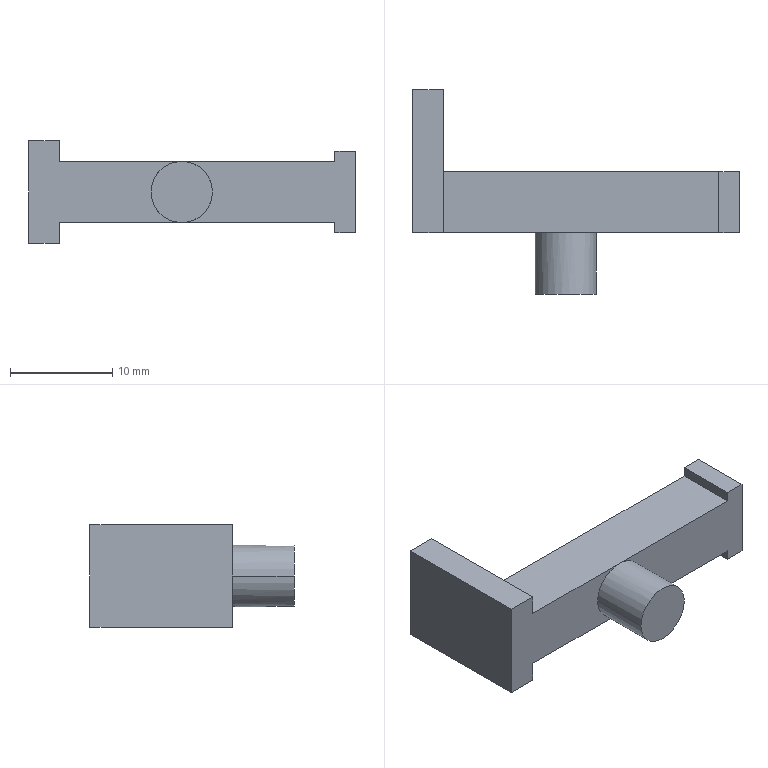Part | SolidWorks | features ICE 5, Extrusion 1 | 1 solid | 18 faces | box 32 x 20 x 10 mm | volume 1658 mm3 | plane 16 | cylinder 2 | commonest cylinder face diameters 6 x2
STEP:
#1=CARTESIAN_POINT('',(-7.,-9.,3.));
#2=VERTEX_POINT('',#1);
#3=CARTESIAN_POINT('',(-13.,-9.,3.));
#4=VERTEX_POINT('',#3);
#5=CARTESIAN_POINT('',(-10.,-9.,3.));
#6=DIRECTION('',(0.,-1.,0.));
#7=DIRECTION('',(1.,0.,0.));
#8=AXIS2_PLACEMENT_3D('',#5,#6,#7);
#9=CIRCLE('',#8,3.);
#10=EDGE_CURVE('',#2,#4,#9,.T.);
#11=ORIENTED_EDGE('',*,*,#10,.F.);
#12=CARTESIAN_POINT('',(-7.,-3.,3.));
#13=VERTEX_POINT('',#12);
#14=CARTESIAN_POINT('',(-7.,-9.,3.));
#15=DIRECTION('',(0.,1.,0.));
#16=VECTOR('',#15,1000.);
#17=LINE('',#14,#16);
#18=EDGE_CURVE('',#2,#13,#17,.T.);
#19=ORIENTED_EDGE('',*,*,#18,.T.);
#20=CARTESIAN_POINT('',(-10.,-3.,6.));
#21=VERTEX_POINT('',#20);
#22=CARTESIAN_POINT('',(-10.,-3.,3.));
#23=DIRECTION('',(0.,-1.,0.));
#24=DIRECTION('',(1.,0.,0.));
#25=AXIS2_PLACEMENT_3D('',#22,#23,#24);
#26=CIRCLE('',#25,3.);
#27=EDGE_CURVE('',#13,#21,#26,.T.);
#28=ORIENTED_EDGE('',*,*,#27,.T.);
#29=CARTESIAN_POINT('',(-13.,-3.,3.));
#30=VERTEX_POINT('',#29);
#31=CARTESIAN_POINT('',(-10.,-3.,3.));
#32=DIRECTION('',(0.,-1.,0.));
#33=DIRECTION('',(1.,0.,0.));
#34=AXIS2_PLACEMENT_3D('',#31,#32,#33);
#35=CIRCLE('',#34,3.);
#36=EDGE_CURVE('',#21,#30,#35,.T.);
#37=ORIENTED_EDGE('',*,*,#36,.T.);
#38=CARTESIAN_POINT('',(-13.,-9.,3.));
#39=DIRECTION('',(0.,1.,0.));
#40=VECTOR('',#39,1000.);
#41=LINE('',#38,#40);
#42=EDGE_CURVE('',#4,#30,#41,.T.);
#43=ORIENTED_EDGE('',*,*,#42,.F.);
#44=EDGE_LOOP('',(#11,#19,#28,#37,#43));
#45=FACE_OUTER_BOUND('',#44,.T.);
#46=CARTESIAN_POINT('',(-10.,-9.,3.));
#47=DIRECTION('',(0.,1.,0.));
#48=DIRECTION('',(-1.,0.,0.));
#49=AXIS2_PLACEMENT_3D('',#46,#47,#48);
#50=CYLINDRICAL_SURFACE('',#49,3.);
#51=ADVANCED_FACE('',(#45),#50,.T.);
#52=CARTESIAN_POINT('',(-22.,3.,6.));
#53=VERTEX_POINT('',#52);
#54=CARTESIAN_POINT('',(-22.,3.,0.));
#55=VERTEX_POINT('',#54);
#56=CARTESIAN_POINT('',(-22.,3.,-2.));
#57=DIRECTION('',(0.,0.,-1.));
#58=VECTOR('',#57,1000.);
#59=LINE('',#56,#58);
#60=EDGE_CURVE('',#53,#55,#59,.T.);
#61=ORIENTED_EDGE('',*,*,#60,.F.);
#62=CARTESIAN_POINT('',(5.,3.,6.));
#63=VERTEX_POINT('',#62);
#64=CARTESIAN_POINT('',(25.,3.,6.));
#65=DIRECTION('',(-1.,0.,0.));
#66=VECTOR('',#65,1000.);
#67=LINE('',#64,#66);
#68=EDGE_CURVE('',#63,#53,#67,.T.);
#69=ORIENTED_EDGE('',*,*,#68,.F.);
#70=CARTESIAN_POINT('',(5.,3.,7.));
#71=VERTEX_POINT('',#70);
#72=CARTESIAN_POINT('',(5.,3.,7.));
#73=DIRECTION('',(0.,0.,1.));
#74=VECTOR('',#73,1000.);
#75=LINE('',#72,#74);
#76=EDGE_CURVE('',#63,#71,#75,.T.);
#77=ORIENTED_EDGE('',*,*,#76,.T.);
#78=CARTESIAN_POINT('',(7.,3.,7.));
#79=VERTEX_POINT('',#78);
#80=CARTESIAN_POINT('',(7.,3.,7.));
#81=DIRECTION('',(-1.,0.,0.));
#82=VECTOR('',#81,1000.);
#83=LINE('',#80,#82);
#84=EDGE_CURVE('',#79,#71,#83,.T.);
#85=ORIENTED_EDGE('',*,*,#84,.F.);
#86=CARTESIAN_POINT('',(7.,3.,-1.));
#87=VERTEX_POINT('',#86);
#88=CARTESIAN_POINT('',(7.,3.,7.));
#89=DIRECTION('',(0.,0.,1.));
#90=VECTOR('',#89,1000.);
#91=LINE('',#88,#90);
#92=EDGE_CURVE('',#87,#79,#91,.T.);
#93=ORIENTED_EDGE('',*,*,#92,.F.);
#94=CARTESIAN_POINT('',(5.,3.,-1.));
#95=VERTEX_POINT('',#94);
#96=CARTESIAN_POINT('',(7.,3.,-1.));
#97=DIRECTION('',(-1.,0.,0.));
#98=VECTOR('',#97,1000.);
#99=LINE('',#96,#98);
#100=EDGE_CURVE('',#87,#95,#99,.T.);
#101=ORIENTED_EDGE('',*,*,#100,.T.);
#102=CARTESIAN_POINT('',(5.,3.,0.));
#103=VERTEX_POINT('',#102);
#104=CARTESIAN_POINT('',(5.,3.,7.));
#105=DIRECTION('',(0.,0.,1.));
#106=VECTOR('',#105,1000.);
#107=LINE('',#104,#106);
#108=EDGE_CURVE('',#95,#103,#107,.T.);
#109=ORIENTED_EDGE('',*,*,#108,.T.);
#110=CARTESIAN_POINT('',(25.,3.,0.));
#111=DIRECTION('',(-1.,0.,0.));
#112=VECTOR('',#111,1000.);
#113=LINE('',#110,#112);
#114=EDGE_CURVE('',#103,#55,#113,.T.);
#115=ORIENTED_EDGE('',*,*,#114,.T.);
#116=EDGE_LOOP('',(#61,#69,#77,#85,#93,#101,#109,#115));
#117=FACE_OUTER_BOUND('',#116,.T.);
#118=CARTESIAN_POINT('',(25.,3.,6.));
#119=DIRECTION('',(0.,-1.,0.));
#120=DIRECTION('',(1.,0.,0.));
#121=AXIS2_PLACEMENT_3D('',#118,#119,#120);
#122=PLANE('',#121);
#123=ADVANCED_FACE('',(#117),#122,.F.);
#124=CARTESIAN_POINT('',(5.,-3.,6.));
#125=VERTEX_POINT('',#124);
#126=CARTESIAN_POINT('',(25.,-3.,6.));
#127=DIRECTION('',(1.,0.,0.));
#128=VECTOR('',#127,1000.);
#129=LINE('',#126,#128);
#130=EDGE_CURVE('',#21,#125,#129,.T.);
#131=ORIENTED_EDGE('',*,*,#130,.T.);
#132=CARTESIAN_POINT('',(5.,3.,6.));
#133=DIRECTION('',(0.,-1.,0.));
#134=VECTOR('',#133,1000.);
#135=LINE('',#132,#134);
#136=EDGE_CURVE('',#63,#125,#135,.T.);
#137=ORIENTED_EDGE('',*,*,#136,.F.);
#138=ORIENTED_EDGE('',*,*,#68,.T.);
#139=CARTESIAN_POINT('',(-22.,-3.,6.));
#140=VERTEX_POINT('',#139);
#141=CARTESIAN_POINT('',(-22.,0.,6.));
#142=DIRECTION('',(0.,-1.,0.));
#143=VECTOR('',#142,1000.);
#144=LINE('',#141,#143);
#145=EDGE_CURVE('',#53,#140,#144,.T.);
#146=ORIENTED_EDGE('',*,*,#145,.T.);
#147=CARTESIAN_POINT('',(25.,-3.,6.));
#148=DIRECTION('',(1.,0.,0.));
#149=VECTOR('',#148,1000.);
#150=LINE('',#147,#149);
#151=EDGE_CURVE('',#140,#21,#150,.T.);
#152=ORIENTED_EDGE('',*,*,#151,.T.);
#153=EDGE_LOOP('',(#131,#137,#138,#146,#152));
#154=FACE_OUTER_BOUND('',#153,.T.);
#155=CARTESIAN_POINT('',(0.,0.,6.));
#156=DIRECTION('',(0.,0.,1.));
#157=DIRECTION('',(1.,0.,0.));
#158=AXIS2_PLACEMENT_3D('',#155,#156,#157);
#159=PLANE('',#158);
#160=ADVANCED_FACE('',(#154),#159,.T.);
#161=CARTESIAN_POINT('',(5.,-3.,0.));
#162=VERTEX_POINT('',#161);
#163=CARTESIAN_POINT('',(5.,-3.,0.));
#164=DIRECTION('',(0.,1.,0.));
#165=VECTOR('',#164,1000.);
#166=LINE('',#163,#165);
#167=EDGE_CURVE('',#162,#103,#166,.T.);
#168=ORIENTED_EDGE('',*,*,#167,.F.);
#169=CARTESIAN_POINT('',(-10.,-3.,0.));
#170=VERTEX_POINT('',#169);
#171=CARTESIAN_POINT('',(25.,-3.,0.));
#172=DIRECTION('',(1.,0.,0.));
#173=VECTOR('',#172,1000.);
#174=LINE('',#171,#173);
#175=EDGE_CURVE('',#170,#162,#174,.T.);
#176=ORIENTED_EDGE('',*,*,#175,.F.);
#177=CARTESIAN_POINT('',(-22.,-3.,0.));
#178=VERTEX_POINT('',#177);
#179=CARTESIAN_POINT('',(25.,-3.,0.));
#180=DIRECTION('',(1.,0.,0.));
#181=VECTOR('',#180,1000.);
#182=LINE('',#179,#181);
#183=EDGE_CURVE('',#178,#170,#182,.T.);
#184=ORIENTED_EDGE('',*,*,#183,.F.);
#185=CARTESIAN_POINT('',(-22.,0.,0.));
#186=DIRECTION('',(0.,-1.,0.));
#187=VECTOR('',#186,1000.);
#188=LINE('',#185,#187);
#189=EDGE_CURVE('',#55,#178,#188,.T.);
#190=ORIENTED_EDGE('',*,*,#189,.F.);
#191=ORIENTED_EDGE('',*,*,#114,.F.);
#192=EDGE_LOOP('',(#168,#176,#184,#190,#191));
#193=FACE_OUTER_BOUND('',#192,.T.);
#194=CARTESIAN_POINT('',(0.,0.,0.));
#195=DIRECTION('',(0.,0.,1.));
#196=DIRECTION('',(1.,0.,0.));
#197=AXIS2_PLACEMENT_3D('',#194,#195,#196);
#198=PLANE('',#197);
#199=ADVANCED_FACE('',(#193),#198,.F.);
#200=ORIENTED_EDGE('',*,*,#175,.T.);
#201=CARTESIAN_POINT('',(5.,-3.,-1.));
#202=VERTEX_POINT('',#201);
#203=CARTESIAN_POINT('',(5.,-3.,7.));
#204=DIRECTION('',(0.,0.,-1.));
#205=VECTOR('',#204,1000.);
#206=LINE('',#203,#205);
#207=EDGE_CURVE('',#162,#202,#206,.T.);
#208=ORIENTED_EDGE('',*,*,#207,.T.);
#209=CARTESIAN_POINT('',(7.,-3.,-1.));
#210=VERTEX_POINT('',#209);
#211=CARTESIAN_POINT('',(7.,-3.,-1.));
#212=DIRECTION('',(-1.,0.,0.));
#213=VECTOR('',#212,1000.);
#214=LINE('',#211,#213);
#215=EDGE_CURVE('',#210,#202,#214,.T.);
#216=ORIENTED_EDGE('',*,*,#215,.F.);
#217=CARTESIAN_POINT('',(7.,-3.,7.));
#218=VERTEX_POINT('',#217);
#219=CARTESIAN_POINT('',(7.,-3.,7.));
#220=DIRECTION('',(0.,0.,-1.));
#221=VECTOR('',#220,1000.);
#222=LINE('',#219,#221);
#223=EDGE_CURVE('',#218,#210,#222,.T.);
#224=ORIENTED_EDGE('',*,*,#223,.F.);
#225=CARTESIAN_POINT('',(5.,-3.,7.));
#226=VERTEX_POINT('',#225);
#227=CARTESIAN_POINT('',(7.,-3.,7.));
#228=DIRECTION('',(-1.,0.,0.));
#229=VECTOR('',#228,1000.);
#230=LINE('',#227,#229);
#231=EDGE_CURVE('',#218,#226,#230,.T.);
#232=ORIENTED_EDGE('',*,*,#231,.T.);
#233=CARTESIAN_POINT('',(5.,-3.,7.));
#234=DIRECTION('',(0.,0.,-1.));
#235=VECTOR('',#234,1000.);
#236=LINE('',#233,#235);
#237=EDGE_CURVE('',#226,#125,#236,.T.);
#238=ORIENTED_EDGE('',*,*,#237,.T.);
#239=ORIENTED_EDGE('',*,*,#130,.F.);
#240=ORIENTED_EDGE('',*,*,#27,.F.);
#241=CARTESIAN_POINT('',(-10.,-3.,3.));
#242=DIRECTION('',(0.,-1.,0.));
#243=DIRECTION('',(1.,0.,0.));
#244=AXIS2_PLACEMENT_3D('',#241,#242,#243);
#245=CIRCLE('',#244,3.);
#246=EDGE_CURVE('',#170,#13,#245,.T.);
#247=ORIENTED_EDGE('',*,*,#246,.F.);
#248=EDGE_LOOP('',(#200,#208,#216,#224,#232,#238,#239,#240,#247));
#249=FACE_OUTER_BOUND('',#248,.T.);
#250=CARTESIAN_POINT('',(25.,-3.,6.));
#251=DIRECTION('',(0.,1.,0.));
#252=DIRECTION('',(-1.,0.,0.));
#253=AXIS2_PLACEMENT_3D('',#250,#251,#252);
#254=PLANE('',#253);
#255=ADVANCED_FACE('',(#249),#254,.F.);
#256=CARTESIAN_POINT('',(-25.,-3.,8.));
#257=VERTEX_POINT('',#256);
#258=CARTESIAN_POINT('',(-25.,-3.,-2.));
#259=VERTEX_POINT('',#258);
#260=CARTESIAN_POINT('',(-25.,-3.,6.));
#261=DIRECTION('',(0.,0.,-1.));
#262=VECTOR('',#261,1000.);
#263=LINE('',#260,#262);
#264=EDGE_CURVE('',#257,#259,#263,.T.);
#265=ORIENTED_EDGE('',*,*,#264,.T.);
#266=CARTESIAN_POINT('',(-22.,-3.,-2.));
#267=VERTEX_POINT('',#266);
#268=CARTESIAN_POINT('',(-22.,-3.,-2.));
#269=DIRECTION('',(-1.,0.,0.));
#270=VECTOR('',#269,1000.);
#271=LINE('',#268,#270);
#272=EDGE_CURVE('',#267,#259,#271,.T.);
#273=ORIENTED_EDGE('',*,*,#272,.F.);
#274=CARTESIAN_POINT('',(-22.,-3.,-2.));
#275=DIRECTION('',(0.,0.,1.));
#276=VECTOR('',#275,1000.);
#277=LINE('',#274,#276);
#278=EDGE_CURVE('',#267,#178,#277,.T.);
#279=ORIENTED_EDGE('',*,*,#278,.T.);
#280=ORIENTED_EDGE('',*,*,#183,.T.);
#281=CARTESIAN_POINT('',(-10.,-3.,3.));
#282=DIRECTION('',(0.,-1.,0.));
#283=DIRECTION('',(1.,0.,0.));
#284=AXIS2_PLACEMENT_3D('',#281,#282,#283);
#285=CIRCLE('',#284,3.);
#286=EDGE_CURVE('',#30,#170,#285,.T.);
#287=ORIENTED_EDGE('',*,*,#286,.F.);
#288=ORIENTED_EDGE('',*,*,#36,.F.);
#289=ORIENTED_EDGE('',*,*,#151,.F.);
#290=CARTESIAN_POINT('',(-22.,-3.,8.));
#291=VERTEX_POINT('',#290);
#292=CARTESIAN_POINT('',(-22.,-3.,-2.));
#293=DIRECTION('',(0.,0.,1.));
#294=VECTOR('',#293,1000.);
#295=LINE('',#292,#294);
#296=EDGE_CURVE('',#140,#291,#295,.T.);
#297=ORIENTED_EDGE('',*,*,#296,.T.);
#298=CARTESIAN_POINT('',(-22.,-3.,8.));
#299=DIRECTION('',(-1.,0.,0.));
#300=VECTOR('',#299,1000.);
#301=LINE('',#298,#300);
#302=EDGE_CURVE('',#291,#257,#301,.T.);
#303=ORIENTED_EDGE('',*,*,#302,.T.);
#304=EDGE_LOOP('',(#265,#273,#279,#280,#287,#288,#289,#297,#303));
#305=FACE_OUTER_BOUND('',#304,.T.);
#306=CARTESIAN_POINT('',(25.,-3.,6.));
#307=DIRECTION('',(0.,1.,0.));
#308=DIRECTION('',(-1.,0.,0.));
#309=AXIS2_PLACEMENT_3D('',#306,#307,#308);
#310=PLANE('',#309);
#311=ADVANCED_FACE('',(#305),#310,.F.);
#312=CARTESIAN_POINT('',(-25.,11.,8.));
#313=VERTEX_POINT('',#312);
#314=CARTESIAN_POINT('',(-25.,3.,8.));
#315=DIRECTION('',(0.,1.,0.));
#316=VECTOR('',#315,1000.);
#317=LINE('',#314,#316);
#318=EDGE_CURVE('',#257,#313,#317,.T.);
#319=ORIENTED_EDGE('',*,*,#318,.T.);
#320=CARTESIAN_POINT('',(-25.,11.,-2.));
#321=VERTEX_POINT('',#320);
#322=CARTESIAN_POINT('',(-25.,11.,-2.));
#323=DIRECTION('',(0.,0.,1.));
#324=VECTOR('',#323,1000.);
#325=LINE('',#322,#324);
#326=EDGE_CURVE('',#321,#313,#325,.T.);
#327=ORIENTED_EDGE('',*,*,#326,.F.);
#328=CARTESIAN_POINT('',(-25.,3.,-2.));
#329=DIRECTION('',(0.,-1.,0.));
#330=VECTOR('',#329,1000.);
#331=LINE('',#328,#330);
#332=EDGE_CURVE('',#321,#259,#331,.T.);
#333=ORIENTED_EDGE('',*,*,#332,.T.);
#334=ORIENTED_EDGE('',*,*,#264,.F.);
#335=EDGE_LOOP('',(#319,#327,#333,#334));
#336=FACE_OUTER_BOUND('',#335,.T.);
#337=CARTESIAN_POINT('',(-25.,-3.,6.));
#338=DIRECTION('',(1.,0.,0.));
#339=DIRECTION('',(0.,0.,-1.));
#340=AXIS2_PLACEMENT_3D('',#337,#338,#339);
#341=PLANE('',#340);
#342=ADVANCED_FACE('',(#336),#341,.F.);
#343=ORIENTED_EDGE('',*,*,#18,.F.);
#344=CARTESIAN_POINT('',(-10.,-9.,3.));
#345=DIRECTION('',(0.,-1.,0.));
#346=DIRECTION('',(1.,0.,0.));
#347=AXIS2_PLACEMENT_3D('',#344,#345,#346);
#348=CIRCLE('',#347,3.);
#349=EDGE_CURVE('',#4,#2,#348,.T.);
#350=ORIENTED_EDGE('',*,*,#349,.F.);
#351=ORIENTED_EDGE('',*,*,#42,.T.);
#352=ORIENTED_EDGE('',*,*,#286,.T.);
#353=ORIENTED_EDGE('',*,*,#246,.T.);
#354=EDGE_LOOP('',(#343,#350,#351,#352,#353));
#355=FACE_OUTER_BOUND('',#354,.T.);
#356=CARTESIAN_POINT('',(-10.,-9.,3.));
#357=DIRECTION('',(0.,1.,0.));
#358=DIRECTION('',(-1.,0.,0.));
#359=AXIS2_PLACEMENT_3D('',#356,#357,#358);
#360=CYLINDRICAL_SURFACE('',#359,3.);
#361=ADVANCED_FACE('',(#355),#360,.T.);
#362=ORIENTED_EDGE('',*,*,#349,.T.);
#363=ORIENTED_EDGE('',*,*,#10,.T.);
#364=EDGE_LOOP('',(#362,#363));
#365=FACE_OUTER_BOUND('',#364,.T.);
#366=CARTESIAN_POINT('',(-10.,-9.,3.));
#367=DIRECTION('',(0.,-1.,0.));
#368=DIRECTION('',(1.,0.,0.));
#369=AXIS2_PLACEMENT_3D('',#366,#367,#368);
#370=PLANE('',#369);
#371=ADVANCED_FACE('',(#365),#370,.T.);
#372=ORIENTED_EDGE('',*,*,#332,.F.);
#373=CARTESIAN_POINT('',(-22.,11.,-2.));
#374=VERTEX_POINT('',#373);
#375=CARTESIAN_POINT('',(-25.,11.,-2.));
#376=DIRECTION('',(-1.,0.,0.));
#377=VECTOR('',#376,1000.);
#378=LINE('',#375,#377);
#379=EDGE_CURVE('',#374,#321,#378,.T.);
#380=ORIENTED_EDGE('',*,*,#379,.F.);
#381=CARTESIAN_POINT('',(-22.,3.,-2.));
#382=DIRECTION('',(0.,-1.,0.));
#383=VECTOR('',#382,1000.);
#384=LINE('',#381,#383);
#385=EDGE_CURVE('',#374,#267,#384,.T.);
#386=ORIENTED_EDGE('',*,*,#385,.T.);
#387=ORIENTED_EDGE('',*,*,#272,.T.);
#388=EDGE_LOOP('',(#372,#380,#386,#387));
#389=FACE_OUTER_BOUND('',#388,.T.);
#390=CARTESIAN_POINT('',(-22.,3.,-2.));
#391=DIRECTION('',(0.,0.,-1.));
#392=DIRECTION('',(0.,1.,0.));
#393=AXIS2_PLACEMENT_3D('',#390,#391,#392);
#394=PLANE('',#393);
#395=ADVANCED_FACE('',(#389),#394,.T.);
#396=ORIENTED_EDGE('',*,*,#385,.F.);
#397=CARTESIAN_POINT('',(-22.,11.,8.));
#398=VERTEX_POINT('',#397);
#399=CARTESIAN_POINT('',(-22.,11.,-2.));
#400=DIRECTION('',(0.,0.,-1.));
#401=VECTOR('',#400,1000.);
#402=LINE('',#399,#401);
#403=EDGE_CURVE('',#398,#374,#402,.T.);
#404=ORIENTED_EDGE('',*,*,#403,.F.);
#405=CARTESIAN_POINT('',(-22.,3.,8.));
#406=DIRECTION('',(0.,1.,0.));
#407=VECTOR('',#406,1000.);
#408=LINE('',#405,#407);
#409=EDGE_CURVE('',#291,#398,#408,.T.);
#410=ORIENTED_EDGE('',*,*,#409,.F.);
#411=ORIENTED_EDGE('',*,*,#296,.F.);
#412=ORIENTED_EDGE('',*,*,#145,.F.);
#413=ORIENTED_EDGE('',*,*,#60,.T.);
#414=ORIENTED_EDGE('',*,*,#189,.T.);
#415=ORIENTED_EDGE('',*,*,#278,.F.);
#416=EDGE_LOOP('',(#396,#404,#410,#411,#412,#413,#414,#415));
#417=FACE_OUTER_BOUND('',#416,.T.);
#418=CARTESIAN_POINT('',(-22.,0.,0.));
#419=DIRECTION('',(-1.,0.,0.));
#420=DIRECTION('',(0.,0.,1.));
#421=AXIS2_PLACEMENT_3D('',#418,#419,#420);
#422=PLANE('',#421);
#423=ADVANCED_FACE('',(#417),#422,.F.);
#424=ORIENTED_EDGE('',*,*,#318,.F.);
#425=ORIENTED_EDGE('',*,*,#302,.F.);
#426=ORIENTED_EDGE('',*,*,#409,.T.);
#427=CARTESIAN_POINT('',(-25.,11.,8.));
#428=DIRECTION('',(1.,0.,0.));
#429=VECTOR('',#428,1000.);
#430=LINE('',#427,#429);
#431=EDGE_CURVE('',#313,#398,#430,.T.);
#432=ORIENTED_EDGE('',*,*,#431,.F.);
#433=EDGE_LOOP('',(#424,#425,#426,#432));
#434=FACE_OUTER_BOUND('',#433,.T.);
#435=CARTESIAN_POINT('',(-22.,3.,8.));
#436=DIRECTION('',(0.,0.,1.));
#437=DIRECTION('',(1.,0.,0.));
#438=AXIS2_PLACEMENT_3D('',#435,#436,#437);
#439=PLANE('',#438);
#440=ADVANCED_FACE('',(#434),#439,.T.);
#441=ORIENTED_EDGE('',*,*,#207,.F.);
#442=ORIENTED_EDGE('',*,*,#167,.T.);
#443=ORIENTED_EDGE('',*,*,#108,.F.);
#444=CARTESIAN_POINT('',(5.,3.,-1.));
#445=DIRECTION('',(0.,1.,0.));
#446=VECTOR('',#445,1000.);
#447=LINE('',#444,#446);
#448=EDGE_CURVE('',#202,#95,#447,.T.);
#449=ORIENTED_EDGE('',*,*,#448,.F.);
#450=EDGE_LOOP('',(#441,#442,#443,#449));
#451=FACE_OUTER_BOUND('',#450,.T.);
#452=CARTESIAN_POINT('',(5.,0.,0.));
#453=DIRECTION('',(1.,0.,0.));
#454=DIRECTION('',(0.,0.,-1.));
#455=AXIS2_PLACEMENT_3D('',#452,#453,#454);
#456=PLANE('',#455);
#457=ADVANCED_FACE('',(#451),#456,.F.);
#458=ORIENTED_EDGE('',*,*,#76,.F.);
#459=ORIENTED_EDGE('',*,*,#136,.T.);
#460=ORIENTED_EDGE('',*,*,#237,.F.);
#461=CARTESIAN_POINT('',(5.,3.,7.));
#462=DIRECTION('',(0.,-1.,0.));
#463=VECTOR('',#462,1000.);
#464=LINE('',#461,#463);
#465=EDGE_CURVE('',#71,#226,#464,.T.);
#466=ORIENTED_EDGE('',*,*,#465,.F.);
#467=EDGE_LOOP('',(#458,#459,#460,#466));
#468=FACE_OUTER_BOUND('',#467,.T.);
#469=CARTESIAN_POINT('',(5.,0.,0.));
#470=DIRECTION('',(1.,0.,0.));
#471=DIRECTION('',(0.,0.,-1.));
#472=AXIS2_PLACEMENT_3D('',#469,#470,#471);
#473=PLANE('',#472);
#474=ADVANCED_FACE('',(#468),#473,.F.);
#475=ORIENTED_EDGE('',*,*,#448,.T.);
#476=ORIENTED_EDGE('',*,*,#100,.F.);
#477=CARTESIAN_POINT('',(7.,3.,-1.));
#478=DIRECTION('',(0.,1.,0.));
#479=VECTOR('',#478,1000.);
#480=LINE('',#477,#479);
#481=EDGE_CURVE('',#210,#87,#480,.T.);
#482=ORIENTED_EDGE('',*,*,#481,.F.);
#483=ORIENTED_EDGE('',*,*,#215,.T.);
#484=EDGE_LOOP('',(#475,#476,#482,#483));
#485=FACE_OUTER_BOUND('',#484,.T.);
#486=CARTESIAN_POINT('',(7.,3.,-1.));
#487=DIRECTION('',(0.,0.,1.));
#488=DIRECTION('',(1.,0.,0.));
#489=AXIS2_PLACEMENT_3D('',#486,#487,#488);
#490=PLANE('',#489);
#491=ADVANCED_FACE('',(#485),#490,.F.);
#492=ORIENTED_EDGE('',*,*,#465,.T.);
#493=ORIENTED_EDGE('',*,*,#231,.F.);
#494=CARTESIAN_POINT('',(7.,3.,7.));
#495=DIRECTION('',(0.,-1.,0.));
#496=VECTOR('',#495,1000.);
#497=LINE('',#494,#496);
#498=EDGE_CURVE('',#79,#218,#497,.T.);
#499=ORIENTED_EDGE('',*,*,#498,.F.);
#500=ORIENTED_EDGE('',*,*,#84,.T.);
#501=EDGE_LOOP('',(#492,#493,#499,#500));
#502=FACE_OUTER_BOUND('',#501,.T.);
#503=CARTESIAN_POINT('',(7.,3.,7.));
#504=DIRECTION('',(0.,0.,-1.));
#505=DIRECTION('',(-1.,0.,0.));
#506=AXIS2_PLACEMENT_3D('',#503,#504,#505);
#507=PLANE('',#506);
#508=ADVANCED_FACE('',(#502),#507,.F.);
#509=ORIENTED_EDGE('',*,*,#481,.T.);
#510=ORIENTED_EDGE('',*,*,#92,.T.);
#511=ORIENTED_EDGE('',*,*,#498,.T.);
#512=ORIENTED_EDGE('',*,*,#223,.T.);
#513=EDGE_LOOP('',(#509,#510,#511,#512));
#514=FACE_OUTER_BOUND('',#513,.T.);
#515=CARTESIAN_POINT('',(7.,0.,0.));
#516=DIRECTION('',(1.,0.,0.));
#517=DIRECTION('',(0.,0.,-1.));
#518=AXIS2_PLACEMENT_3D('',#515,#516,#517);
#519=PLANE('',#518);
#520=ADVANCED_FACE('',(#514),#519,.T.);
#521=ORIENTED_EDGE('',*,*,#326,.T.);
#522=ORIENTED_EDGE('',*,*,#431,.T.);
#523=ORIENTED_EDGE('',*,*,#403,.T.);
#524=ORIENTED_EDGE('',*,*,#379,.T.);
#525=EDGE_LOOP('',(#521,#522,#523,#524));
#526=FACE_OUTER_BOUND('',#525,.T.);
#527=CARTESIAN_POINT('',(0.,11.,0.));
#528=DIRECTION('',(0.,1.,0.));
#529=DIRECTION('',(-1.,0.,0.));
#530=AXIS2_PLACEMENT_3D('',#527,#528,#529);
#531=PLANE('',#530);
#532=ADVANCED_FACE('',(#526),#531,.T.);
#533=CLOSED_SHELL('',(#51,#123,#160,#199,#255,#311,#342,#361,#371,#395,#423,#440,#457,#474,#491,#508,#520,#532));
#534=MANIFOLD_SOLID_BREP('',#533);
#535=CARTESIAN_POINT('',(0.,0.,0.));
#536=DIRECTION('',(0.,0.,1.));
#537=DIRECTION('',(1.,0.,0.));
#538=AXIS2_PLACEMENT_3D('',#535,#536,#537);
#539=(LENGTH_UNIT()NAMED_UNIT(*)SI_UNIT(.MILLI.,.METRE.));
#540=UNCERTAINTY_MEASURE_WITH_UNIT(LENGTH_MEASURE(0.00001),#539,'','');
#541=(NAMED_UNIT(*)PLANE_ANGLE_UNIT()SI_UNIT($,.RADIAN.));
#542=(NAMED_UNIT(*)SI_UNIT($,.STERADIAN.)SOLID_ANGLE_UNIT());
#543=(GEOMETRIC_REPRESENTATION_CONTEXT(3)GLOBAL_UNCERTAINTY_ASSIGNED_CONTEXT((#540))GLOBAL_UNIT_ASSIGNED_CONTEXT((#539,#541,#542))REPRESENTATION_CONTEXT('',''));
#544=ADVANCED_BREP_SHAPE_REPRESENTATION('',(#534,#538),#543);